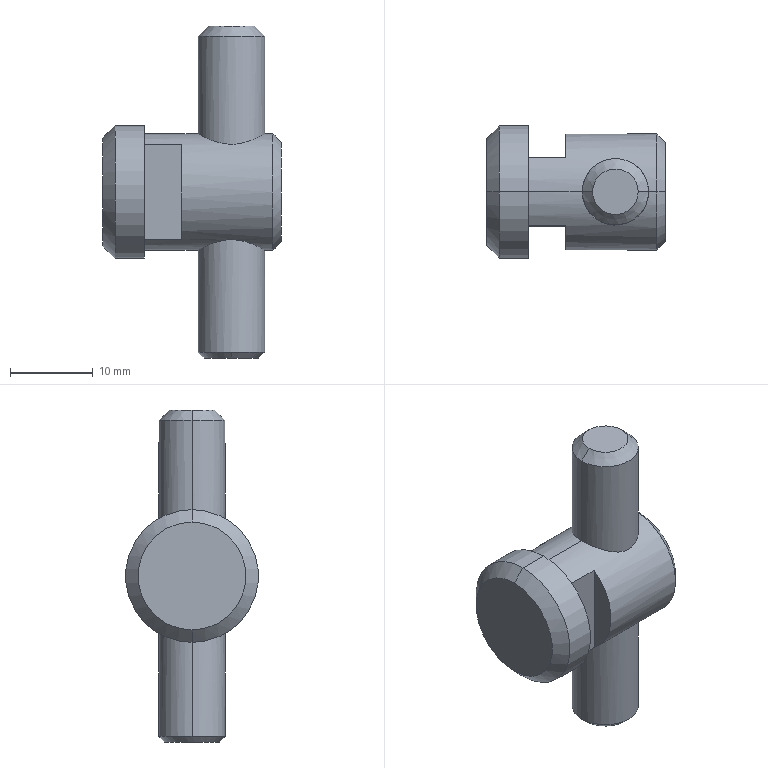Part | SolidWorks | features BaseBody 3, ICE 1 | 1 solid | 39 faces | box 21.5 x 16 x 40 mm | volume 4531 mm3 | plane 21 | cone 10 | cylinder 8 | commonest cylinder face diameters 8 x4 14 x2 16 x2
STEP:
#1=CARTESIAN_POINT('',(17.561,-2.765,31.125));
#2=VERTEX_POINT('',#1);
#3=CARTESIAN_POINT('',(25.561,-2.765,31.125));
#4=VERTEX_POINT('',#3);
#5=CARTESIAN_POINT('',(21.561,-2.765,31.125));
#6=DIRECTION('',(0.,0.,-1.));
#7=DIRECTION('',(-1.,0.,0.));
#8=AXIS2_PLACEMENT_3D('',#5,#6,#7);
#9=CIRCLE('',#8,4.);
#10=EDGE_CURVE('',#2,#4,#9,.T.);
#11=ORIENTED_EDGE('',*,*,#10,.T.);
#12=CARTESIAN_POINT('',(25.561,-2.765,19.375));
#13=VERTEX_POINT('',#12);
#14=CARTESIAN_POINT('',(25.561,-2.765,-18.37));
#15=DIRECTION('',(0.,0.,-1.));
#16=VECTOR('',#15,1000.);
#17=LINE('',#14,#16);
#18=EDGE_CURVE('',#4,#13,#17,.T.);
#19=ORIENTED_EDGE('',*,*,#18,.T.);
#20=CARTESIAN_POINT('',(17.561,-2.765,19.375));
#21=VERTEX_POINT('',#20);
#22=CARTESIAN_POINT('',(17.561,-2.765,19.375));
#23=CARTESIAN_POINT('',(17.561,-2.494,19.375));
#24=CARTESIAN_POINT('',(17.588,-2.229,19.359));
#25=CARTESIAN_POINT('',(17.694,-1.709,19.3));
#26=CARTESIAN_POINT('',(17.774,-1.452,19.255));
#27=CARTESIAN_POINT('',(17.977,-0.9687,19.145));
#28=CARTESIAN_POINT('',(18.101,-0.7408,19.08));
#29=CARTESIAN_POINT('',(18.392,-0.3103,18.934));
#30=CARTESIAN_POINT('',(18.556,-0.1123,18.856));
#31=CARTESIAN_POINT('',(18.917,0.2479,18.697));
#32=CARTESIAN_POINT('',(19.117,0.4123,18.615));
#33=CARTESIAN_POINT('',(19.544,0.6988,18.46));
#34=CARTESIAN_POINT('',(19.769,0.8207,18.388));
#35=CARTESIAN_POINT('',(20.247,1.022,18.263));
#36=CARTESIAN_POINT('',(20.503,1.102,18.21));
#37=CARTESIAN_POINT('',(21.023,1.208,18.139));
#38=CARTESIAN_POINT('',(21.289,1.235,18.12));
#39=CARTESIAN_POINT('',(21.831,1.235,18.12));
#40=CARTESIAN_POINT('',(22.096,1.208,18.139));
#41=CARTESIAN_POINT('',(22.616,1.103,18.21));
#42=CARTESIAN_POINT('',(22.872,1.023,18.263));
#43=CARTESIAN_POINT('',(23.352,0.8211,18.388));
#44=CARTESIAN_POINT('',(23.582,0.6969,18.461));
#45=CARTESIAN_POINT('',(24.009,0.4088,18.616));
#46=CARTESIAN_POINT('',(24.206,0.2466,18.697));
#47=CARTESIAN_POINT('',(24.568,-0.1149,18.857));
#48=CARTESIAN_POINT('',(24.734,-0.3159,18.937));
#49=CARTESIAN_POINT('',(25.021,-0.7423,19.08));
#50=CARTESIAN_POINT('',(25.145,-0.9692,19.145));
#51=CARTESIAN_POINT('',(25.298,-1.332,19.228));
#52=CARTESIAN_POINT('',(25.344,-1.458,19.253));
#53=CARTESIAN_POINT('',(25.422,-1.711,19.296));
#54=CARTESIAN_POINT('',(25.455,-1.84,19.315));
#55=CARTESIAN_POINT('',(25.534,-2.229,19.359));
#56=CARTESIAN_POINT('',(25.561,-2.494,19.375));
#57=CARTESIAN_POINT('',(25.561,-2.765,19.375));
#58=B_SPLINE_CURVE_WITH_KNOTS('',3,(#22,#23,#24,#25,#26,#27,#28,#29,#30,#31,#32,#33,#34,#35,#36,#37,#38,#39,#40,#41,#42,#43,#44,#45,#46,#47,#48,#49,#50,#51,#52,#53,#54,#55,#56,#57),.UNSPECIFIED.,.F.,.F.,(4,2,2,2,2,2,2,2,2,2,2,2,2,2,2,2,2,4),(0.,0.0007999,0.0016,0.0024,0.003199,0.003999,0.004799,0.005599,0.006399,0.007199,0.007999,0.008798,0.009598,0.0104,0.0112,0.0116,0.012,0.0128),.UNSPECIFIED.);
#59=EDGE_CURVE('',#21,#13,#58,.T.);
#60=ORIENTED_EDGE('',*,*,#59,.F.);
#61=CARTESIAN_POINT('',(17.561,-2.765,-18.37));
#62=DIRECTION('',(0.,0.,-1.));
#63=VECTOR('',#62,1000.);
#64=LINE('',#61,#63);
#65=EDGE_CURVE('',#2,#21,#64,.T.);
#66=ORIENTED_EDGE('',*,*,#65,.F.);
#67=EDGE_LOOP('',(#11,#19,#60,#66));
#68=FACE_OUTER_BOUND('',#67,.T.);
#69=CARTESIAN_POINT('',(21.561,-2.765,-18.37));
#70=DIRECTION('',(0.,0.,-1.));
#71=DIRECTION('',(-1.,0.,0.));
#72=AXIS2_PLACEMENT_3D('',#69,#70,#71);
#73=CYLINDRICAL_SURFACE('',#72,4.);
#74=ADVANCED_FACE('',(#68),#73,.T.);
#75=CARTESIAN_POINT('',(18.811,-2.765,32.375));
#76=VERTEX_POINT('',#75);
#77=CARTESIAN_POINT('',(24.311,-2.765,32.375));
#78=VERTEX_POINT('',#77);
#79=CARTESIAN_POINT('',(21.561,-2.765,32.375));
#80=DIRECTION('',(0.,0.,-1.));
#81=DIRECTION('',(-1.,0.,0.));
#82=AXIS2_PLACEMENT_3D('',#79,#80,#81);
#83=CIRCLE('',#82,2.75);
#84=EDGE_CURVE('',#76,#78,#83,.T.);
#85=ORIENTED_EDGE('',*,*,#84,.T.);
#86=CARTESIAN_POINT('',(25.561,-2.765,31.125));
#87=DIRECTION('',(0.7071,0.,-0.7071));
#88=VECTOR('',#87,1000.);
#89=LINE('',#86,#88);
#90=EDGE_CURVE('',#78,#4,#89,.T.);
#91=ORIENTED_EDGE('',*,*,#90,.T.);
#92=ORIENTED_EDGE('',*,*,#10,.F.);
#93=CARTESIAN_POINT('',(17.561,-2.765,31.125));
#94=DIRECTION('',(-0.7071,0.,-0.7071));
#95=VECTOR('',#94,1000.);
#96=LINE('',#93,#95);
#97=EDGE_CURVE('',#76,#2,#96,.T.);
#98=ORIENTED_EDGE('',*,*,#97,.F.);
#99=EDGE_LOOP('',(#85,#91,#92,#98));
#100=FACE_OUTER_BOUND('',#99,.T.);
#101=CARTESIAN_POINT('',(21.561,-2.765,31.125));
#102=DIRECTION('',(0.,0.,-1.));
#103=DIRECTION('',(-1.,0.,0.));
#104=AXIS2_PLACEMENT_3D('',#101,#102,#103);
#105=CONICAL_SURFACE('',#104,4.,0.7854);
#106=ADVANCED_FACE('',(#100),#105,.T.);
#107=CARTESIAN_POINT('',(26.561,-2.765,19.375));
#108=VERTEX_POINT('',#107);
#109=CARTESIAN_POINT('',(26.561,-2.765,5.375));
#110=VERTEX_POINT('',#109);
#111=CARTESIAN_POINT('',(26.561,-2.765,12.375));
#112=DIRECTION('',(-1.,0.,0.));
#113=DIRECTION('',(0.,0.,1.));
#114=AXIS2_PLACEMENT_3D('',#111,#112,#113);
#115=CIRCLE('',#114,7.);
#116=EDGE_CURVE('',#108,#110,#115,.T.);
#117=ORIENTED_EDGE('',*,*,#116,.T.);
#118=CARTESIAN_POINT('',(25.561,-2.765,5.375));
#119=VERTEX_POINT('',#118);
#120=CARTESIAN_POINT('',(27.561,-2.765,5.375));
#121=DIRECTION('',(-1.,0.,0.));
#122=VECTOR('',#121,1000.);
#123=LINE('',#120,#122);
#124=EDGE_CURVE('',#110,#119,#123,.T.);
#125=ORIENTED_EDGE('',*,*,#124,.T.);
#126=CARTESIAN_POINT('',(17.561,-2.765,5.375));
#127=VERTEX_POINT('',#126);
#128=CARTESIAN_POINT('',(25.561,-2.765,5.375));
#129=CARTESIAN_POINT('',(25.561,-2.494,5.375));
#130=CARTESIAN_POINT('',(25.534,-2.229,5.391));
#131=CARTESIAN_POINT('',(25.428,-1.709,5.45));
#132=CARTESIAN_POINT('',(25.348,-1.452,5.495));
#133=CARTESIAN_POINT('',(25.145,-0.9692,5.605));
#134=CARTESIAN_POINT('',(25.021,-0.7408,5.67));
#135=CARTESIAN_POINT('',(24.73,-0.3098,5.816));
#136=CARTESIAN_POINT('',(24.566,-0.1129,5.894));
#137=CARTESIAN_POINT('',(24.205,0.2473,6.053));
#138=CARTESIAN_POINT('',(24.005,0.412,6.135));
#139=CARTESIAN_POINT('',(23.58,0.6978,6.289));
#140=CARTESIAN_POINT('',(23.355,0.8199,6.361));
#141=CARTESIAN_POINT('',(22.876,1.022,6.486));
#142=CARTESIAN_POINT('',(22.62,1.101,6.539));
#143=CARTESIAN_POINT('',(22.101,1.207,6.611));
#144=CARTESIAN_POINT('',(21.833,1.235,6.63));
#145=CARTESIAN_POINT('',(21.294,1.235,6.631));
#146=CARTESIAN_POINT('',(21.029,1.209,6.612));
#147=CARTESIAN_POINT('',(20.508,1.103,6.54));
#148=CARTESIAN_POINT('',(20.253,1.024,6.488));
#149=CARTESIAN_POINT('',(19.773,0.8228,6.363));
#150=CARTESIAN_POINT('',(19.543,0.6984,6.29));
#151=CARTESIAN_POINT('',(19.116,0.4115,6.135));
#152=CARTESIAN_POINT('',(18.919,0.2497,6.054));
#153=CARTESIAN_POINT('',(18.556,-0.1119,5.894));
#154=CARTESIAN_POINT('',(18.391,-0.3121,5.815));
#155=CARTESIAN_POINT('',(18.103,-0.7374,5.671));
#156=CARTESIAN_POINT('',(17.979,-0.964,5.606));
#157=CARTESIAN_POINT('',(17.774,-1.449,5.495));
#158=CARTESIAN_POINT('',(17.695,-1.704,5.451));
#159=CARTESIAN_POINT('',(17.589,-2.224,5.391));
#160=CARTESIAN_POINT('',(17.561,-2.495,5.375));
#161=CARTESIAN_POINT('',(17.561,-2.765,5.375));
#162=B_SPLINE_CURVE_WITH_KNOTS('',3,(#128,#129,#130,#131,#132,#133,#134,#135,#136,#137,#138,#139,#140,#141,#142,#143,#144,#145,#146,#147,#148,#149,#150,#151,#152,#153,#154,#155,#156,#157,#158,#159,#160,#161),.UNSPECIFIED.,.F.,.F.,(4,2,2,2,2,2,2,2,2,2,2,2,2,2,2,2,4),(0.0128,0.0136,0.01439,0.01519,0.01599,0.01679,0.01759,0.01838,0.01918,0.01998,0.02078,0.02158,0.02238,0.02317,0.02397,0.02477,0.02557),.UNSPECIFIED.);
#163=EDGE_CURVE('',#119,#127,#162,.T.);
#164=ORIENTED_EDGE('',*,*,#163,.T.);
#165=CARTESIAN_POINT('',(11.061,-2.765,5.375));
#166=VERTEX_POINT('',#165);
#167=CARTESIAN_POINT('',(27.561,-2.765,5.375));
#168=DIRECTION('',(-1.,0.,0.));
#169=VECTOR('',#168,1000.);
#170=LINE('',#167,#169);
#171=EDGE_CURVE('',#127,#166,#170,.T.);
#172=ORIENTED_EDGE('',*,*,#171,.T.);
#173=CARTESIAN_POINT('',(11.061,1.335,6.701));
#174=VERTEX_POINT('',#173);
#175=CARTESIAN_POINT('',(11.061,-2.765,12.375));
#176=DIRECTION('',(1.,0.,0.));
#177=DIRECTION('',(0.,0.,1.));
#178=AXIS2_PLACEMENT_3D('',#175,#176,#177);
#179=CIRCLE('',#178,7.);
#180=EDGE_CURVE('',#166,#174,#179,.T.);
#181=ORIENTED_EDGE('',*,*,#180,.T.);
#182=CARTESIAN_POINT('',(15.561,1.335,6.701));
#183=VERTEX_POINT('',#182);
#184=CARTESIAN_POINT('',(27.561,1.335,6.701));
#185=DIRECTION('',(1.,0.,0.));
#186=VECTOR('',#185,1000.);
#187=LINE('',#184,#186);
#188=EDGE_CURVE('',#174,#183,#187,.T.);
#189=ORIENTED_EDGE('',*,*,#188,.T.);
#190=CARTESIAN_POINT('',(15.561,1.335,18.049));
#191=VERTEX_POINT('',#190);
#192=CARTESIAN_POINT('',(15.561,-2.765,12.375));
#193=DIRECTION('',(1.,0.,0.));
#194=DIRECTION('',(0.,0.,1.));
#195=AXIS2_PLACEMENT_3D('',#192,#193,#194);
#196=CIRCLE('',#195,7.);
#197=EDGE_CURVE('',#183,#191,#196,.T.);
#198=ORIENTED_EDGE('',*,*,#197,.T.);
#199=CARTESIAN_POINT('',(11.061,1.335,18.049));
#200=VERTEX_POINT('',#199);
#201=CARTESIAN_POINT('',(27.561,1.335,18.049));
#202=DIRECTION('',(-1.,0.,0.));
#203=VECTOR('',#202,1000.);
#204=LINE('',#201,#203);
#205=EDGE_CURVE('',#191,#200,#204,.T.);
#206=ORIENTED_EDGE('',*,*,#205,.T.);
#207=CARTESIAN_POINT('',(11.061,-2.765,19.375));
#208=VERTEX_POINT('',#207);
#209=CARTESIAN_POINT('',(11.061,-2.765,12.375));
#210=DIRECTION('',(1.,0.,0.));
#211=DIRECTION('',(0.,0.,1.));
#212=AXIS2_PLACEMENT_3D('',#209,#210,#211);
#213=CIRCLE('',#212,7.);
#214=EDGE_CURVE('',#200,#208,#213,.T.);
#215=ORIENTED_EDGE('',*,*,#214,.T.);
#216=CARTESIAN_POINT('',(27.561,-2.765,19.375));
#217=DIRECTION('',(-1.,0.,0.));
#218=VECTOR('',#217,1000.);
#219=LINE('',#216,#218);
#220=EDGE_CURVE('',#21,#208,#219,.T.);
#221=ORIENTED_EDGE('',*,*,#220,.F.);
#222=ORIENTED_EDGE('',*,*,#59,.T.);
#223=CARTESIAN_POINT('',(27.561,-2.765,19.375));
#224=DIRECTION('',(-1.,0.,0.));
#225=VECTOR('',#224,1000.);
#226=LINE('',#223,#225);
#227=EDGE_CURVE('',#108,#13,#226,.T.);
#228=ORIENTED_EDGE('',*,*,#227,.F.);
#229=EDGE_LOOP('',(#117,#125,#164,#172,#181,#189,#198,#206,#215,#221,#222,#228));
#230=FACE_OUTER_BOUND('',#229,.T.);
#231=CARTESIAN_POINT('',(27.561,-2.765,12.375));
#232=DIRECTION('',(-1.,0.,0.));
#233=DIRECTION('',(0.,0.,1.));
#234=AXIS2_PLACEMENT_3D('',#231,#232,#233);
#235=CYLINDRICAL_SURFACE('',#234,7.);
#236=ADVANCED_FACE('',(#230),#235,.T.);
#237=CARTESIAN_POINT('',(27.561,-2.765,18.375));
#238=VERTEX_POINT('',#237);
#239=CARTESIAN_POINT('',(27.561,-2.765,6.375));
#240=VERTEX_POINT('',#239);
#241=CARTESIAN_POINT('',(27.561,-2.765,12.375));
#242=DIRECTION('',(-1.,0.,0.));
#243=DIRECTION('',(0.,0.,1.));
#244=AXIS2_PLACEMENT_3D('',#241,#242,#243);
#245=CIRCLE('',#244,6.);
#246=EDGE_CURVE('',#238,#240,#245,.T.);
#247=ORIENTED_EDGE('',*,*,#246,.T.);
#248=CARTESIAN_POINT('',(26.561,-2.765,5.375));
#249=DIRECTION('',(-0.7071,0.,-0.7071));
#250=VECTOR('',#249,1000.);
#251=LINE('',#248,#250);
#252=EDGE_CURVE('',#240,#110,#251,.T.);
#253=ORIENTED_EDGE('',*,*,#252,.T.);
#254=ORIENTED_EDGE('',*,*,#116,.F.);
#255=CARTESIAN_POINT('',(26.561,-2.765,19.375));
#256=DIRECTION('',(-0.7071,0.,0.7071));
#257=VECTOR('',#256,1000.);
#258=LINE('',#255,#257);
#259=EDGE_CURVE('',#238,#108,#258,.T.);
#260=ORIENTED_EDGE('',*,*,#259,.F.);
#261=EDGE_LOOP('',(#247,#253,#254,#260));
#262=FACE_OUTER_BOUND('',#261,.T.);
#263=CARTESIAN_POINT('',(26.561,-2.765,12.375));
#264=DIRECTION('',(-1.,0.,0.));
#265=DIRECTION('',(0.,0.,1.));
#266=AXIS2_PLACEMENT_3D('',#263,#264,#265);
#267=CONICAL_SURFACE('',#266,7.,0.7854);
#268=ADVANCED_FACE('',(#262),#267,.T.);
#269=CARTESIAN_POINT('',(11.061,-2.765,4.375));
#270=VERTEX_POINT('',#269);
#271=CARTESIAN_POINT('',(11.061,-2.765,20.375));
#272=VERTEX_POINT('',#271);
#273=CARTESIAN_POINT('',(11.061,-2.765,12.375));
#274=DIRECTION('',(1.,0.,0.));
#275=DIRECTION('',(0.,0.,1.));
#276=AXIS2_PLACEMENT_3D('',#273,#274,#275);
#277=CIRCLE('',#276,8.);
#278=EDGE_CURVE('',#270,#272,#277,.T.);
#279=ORIENTED_EDGE('',*,*,#278,.F.);
#280=CARTESIAN_POINT('',(7.561,-2.765,4.375));
#281=VERTEX_POINT('',#280);
#282=CARTESIAN_POINT('',(11.061,-2.765,4.375));
#283=DIRECTION('',(-1.,0.,0.));
#284=VECTOR('',#283,1000.);
#285=LINE('',#282,#284);
#286=EDGE_CURVE('',#270,#281,#285,.T.);
#287=ORIENTED_EDGE('',*,*,#286,.T.);
#288=CARTESIAN_POINT('',(7.561,-2.765,20.375));
#289=VERTEX_POINT('',#288);
#290=CARTESIAN_POINT('',(7.561,-2.765,12.375));
#291=DIRECTION('',(1.,0.,0.));
#292=DIRECTION('',(0.,0.,1.));
#293=AXIS2_PLACEMENT_3D('',#290,#291,#292);
#294=CIRCLE('',#293,8.);
#295=EDGE_CURVE('',#281,#289,#294,.T.);
#296=ORIENTED_EDGE('',*,*,#295,.T.);
#297=CARTESIAN_POINT('',(11.061,-2.765,20.375));
#298=DIRECTION('',(-1.,0.,0.));
#299=VECTOR('',#298,1000.);
#300=LINE('',#297,#299);
#301=EDGE_CURVE('',#272,#289,#300,.T.);
#302=ORIENTED_EDGE('',*,*,#301,.F.);
#303=EDGE_LOOP('',(#279,#287,#296,#302));
#304=FACE_OUTER_BOUND('',#303,.T.);
#305=CARTESIAN_POINT('',(11.061,-2.765,12.375));
#306=DIRECTION('',(-1.,0.,0.));
#307=DIRECTION('',(0.,0.,1.));
#308=AXIS2_PLACEMENT_3D('',#305,#306,#307);
#309=CYLINDRICAL_SURFACE('',#308,8.);
#310=ADVANCED_FACE('',(#304),#309,.T.);
#311=CARTESIAN_POINT('',(6.061,-2.765,5.875));
#312=VERTEX_POINT('',#311);
#313=CARTESIAN_POINT('',(6.061,-2.765,18.875));
#314=VERTEX_POINT('',#313);
#315=CARTESIAN_POINT('',(6.061,-2.765,12.375));
#316=DIRECTION('',(1.,0.,0.));
#317=DIRECTION('',(0.,0.,-1.));
#318=AXIS2_PLACEMENT_3D('',#315,#316,#317);
#319=CIRCLE('',#318,6.5);
#320=EDGE_CURVE('',#312,#314,#319,.T.);
#321=ORIENTED_EDGE('',*,*,#320,.T.);
#322=CARTESIAN_POINT('',(7.561,-2.765,20.375));
#323=DIRECTION('',(0.7071,0.,0.7071));
#324=VECTOR('',#323,1000.);
#325=LINE('',#322,#324);
#326=EDGE_CURVE('',#314,#289,#325,.T.);
#327=ORIENTED_EDGE('',*,*,#326,.T.);
#328=ORIENTED_EDGE('',*,*,#295,.F.);
#329=CARTESIAN_POINT('',(7.561,-2.765,4.375));
#330=DIRECTION('',(0.7071,0.,-0.7071));
#331=VECTOR('',#330,1000.);
#332=LINE('',#329,#331);
#333=EDGE_CURVE('',#312,#281,#332,.T.);
#334=ORIENTED_EDGE('',*,*,#333,.F.);
#335=EDGE_LOOP('',(#321,#327,#328,#334));
#336=FACE_OUTER_BOUND('',#335,.T.);
#337=CARTESIAN_POINT('',(7.561,-2.765,12.375));
#338=DIRECTION('',(1.,0.,0.));
#339=DIRECTION('',(0.,0.,-1.));
#340=AXIS2_PLACEMENT_3D('',#337,#338,#339);
#341=CONICAL_SURFACE('',#340,8.,0.7854);
#342=ADVANCED_FACE('',(#336),#341,.T.);
#343=ORIENTED_EDGE('',*,*,#163,.F.);
#344=CARTESIAN_POINT('',(25.561,-2.765,-6.948));
#345=VERTEX_POINT('',#344);
#346=CARTESIAN_POINT('',(25.561,-2.765,-18.37));
#347=DIRECTION('',(0.,0.,-1.));
#348=VECTOR('',#347,1000.);
#349=LINE('',#346,#348);
#350=EDGE_CURVE('',#119,#345,#349,.T.);
#351=ORIENTED_EDGE('',*,*,#350,.T.);
#352=CARTESIAN_POINT('',(21.561,1.235,-6.948));
#353=VERTEX_POINT('',#352);
#354=CARTESIAN_POINT('',(21.561,-2.765,-6.948));
#355=DIRECTION('',(0.,0.,1.));
#356=DIRECTION('',(-1.,0.,0.));
#357=AXIS2_PLACEMENT_3D('',#354,#355,#356);
#358=CIRCLE('',#357,4.);
#359=EDGE_CURVE('',#345,#353,#358,.T.);
#360=ORIENTED_EDGE('',*,*,#359,.T.);
#361=CARTESIAN_POINT('',(17.561,-2.765,-6.948));
#362=VERTEX_POINT('',#361);
#363=CARTESIAN_POINT('',(21.561,-2.765,-6.948));
#364=DIRECTION('',(0.,0.,1.));
#365=DIRECTION('',(-1.,0.,0.));
#366=AXIS2_PLACEMENT_3D('',#363,#364,#365);
#367=CIRCLE('',#366,4.);
#368=EDGE_CURVE('',#353,#362,#367,.T.);
#369=ORIENTED_EDGE('',*,*,#368,.T.);
#370=CARTESIAN_POINT('',(17.561,-2.765,-18.37));
#371=DIRECTION('',(0.,0.,-1.));
#372=VECTOR('',#371,1000.);
#373=LINE('',#370,#372);
#374=EDGE_CURVE('',#127,#362,#373,.T.);
#375=ORIENTED_EDGE('',*,*,#374,.F.);
#376=EDGE_LOOP('',(#343,#351,#360,#369,#375));
#377=FACE_OUTER_BOUND('',#376,.T.);
#378=CARTESIAN_POINT('',(21.561,-2.765,-18.37));
#379=DIRECTION('',(0.,0.,-1.));
#380=DIRECTION('',(-1.,0.,0.));
#381=AXIS2_PLACEMENT_3D('',#378,#379,#380);
#382=CYLINDRICAL_SURFACE('',#381,4.);
#383=ADVANCED_FACE('',(#377),#382,.T.);
#384=CARTESIAN_POINT('',(21.561,-6.088,-7.625));
#385=VERTEX_POINT('',#384);
#386=CARTESIAN_POINT('',(21.561,0.5587,-7.625));
#387=VERTEX_POINT('',#386);
#388=CARTESIAN_POINT('',(21.561,-2.765,-7.625));
#389=DIRECTION('',(0.,0.,1.));
#390=DIRECTION('',(0.,-1.,0.));
#391=AXIS2_PLACEMENT_3D('',#388,#389,#390);
#392=CIRCLE('',#391,3.323);
#393=EDGE_CURVE('',#385,#387,#392,.T.);
#394=ORIENTED_EDGE('',*,*,#393,.T.);
#395=CARTESIAN_POINT('',(21.561,1.235,-6.949));
#396=DIRECTION('',(0.,0.7071,0.7071));
#397=VECTOR('',#396,1000.);
#398=LINE('',#395,#397);
#399=EDGE_CURVE('',#387,#353,#398,.T.);
#400=ORIENTED_EDGE('',*,*,#399,.T.);
#401=ORIENTED_EDGE('',*,*,#359,.F.);
#402=CARTESIAN_POINT('',(21.561,-6.765,-6.948));
#403=VERTEX_POINT('',#402);
#404=CARTESIAN_POINT('',(21.561,-2.765,-6.948));
#405=DIRECTION('',(0.,0.,1.));
#406=DIRECTION('',(-1.,0.,0.));
#407=AXIS2_PLACEMENT_3D('',#404,#405,#406);
#408=CIRCLE('',#407,4.);
#409=EDGE_CURVE('',#403,#345,#408,.T.);
#410=ORIENTED_EDGE('',*,*,#409,.F.);
#411=CARTESIAN_POINT('',(21.561,-6.765,-6.949));
#412=DIRECTION('',(0.,-0.7071,0.7071));
#413=VECTOR('',#412,1000.);
#414=LINE('',#411,#413);
#415=EDGE_CURVE('',#385,#403,#414,.T.);
#416=ORIENTED_EDGE('',*,*,#415,.F.);
#417=EDGE_LOOP('',(#394,#400,#401,#410,#416));
#418=FACE_OUTER_BOUND('',#417,.T.);
#419=CARTESIAN_POINT('',(21.561,-2.765,-6.949));
#420=DIRECTION('',(0.,0.,1.));
#421=DIRECTION('',(0.,-1.,0.));
#422=AXIS2_PLACEMENT_3D('',#419,#420,#421);
#423=CONICAL_SURFACE('',#422,4.,0.7854);
#424=ADVANCED_FACE('',(#418),#423,.T.);
#425=CARTESIAN_POINT('',(21.561,-2.765,-3.47));
#426=VERTEX_POINT('',#425);
#427=CARTESIAN_POINT('',(21.561,-0.7648,-4.625));
#428=VERTEX_POINT('',#427);
#429=CARTESIAN_POINT('',(21.561,-0.7648,-4.625));
#430=DIRECTION('',(0.,0.866,-0.5));
#431=VECTOR('',#430,1000.);
#432=LINE('',#429,#431);
#433=EDGE_CURVE('',#426,#428,#432,.T.);
#434=ORIENTED_EDGE('',*,*,#433,.F.);
#435=CARTESIAN_POINT('',(21.561,-4.765,-4.625));
#436=VERTEX_POINT('',#435);
#437=CARTESIAN_POINT('',(21.561,-4.765,-4.625));
#438=DIRECTION('',(0.,-0.866,-0.5));
#439=VECTOR('',#438,1000.);
#440=LINE('',#437,#439);
#441=EDGE_CURVE('',#426,#436,#440,.T.);
#442=ORIENTED_EDGE('',*,*,#441,.T.);
#443=CARTESIAN_POINT('',(20.212,-4.242,-4.625));
#444=VERTEX_POINT('',#443);
#445=CARTESIAN_POINT('',(21.561,-2.765,-4.625));
#446=DIRECTION('',(0.,0.,-1.));
#447=DIRECTION('',(0.,1.,0.));
#448=AXIS2_PLACEMENT_3D('',#445,#446,#447);
#449=CIRCLE('',#448,2.);
#450=EDGE_CURVE('',#436,#444,#449,.T.);
#451=ORIENTED_EDGE('',*,*,#450,.T.);
#452=CARTESIAN_POINT('',(19.607,-2.335,-4.625));
#453=VERTEX_POINT('',#452);
#454=CARTESIAN_POINT('',(21.561,-2.765,-4.625));
#455=DIRECTION('',(0.,0.,1.));
#456=DIRECTION('',(0.,1.,0.));
#457=AXIS2_PLACEMENT_3D('',#454,#455,#456);
#458=CIRCLE('',#457,2.);
#459=EDGE_CURVE('',#453,#444,#458,.T.);
#460=ORIENTED_EDGE('',*,*,#459,.F.);
#461=CARTESIAN_POINT('',(20.956,-0.8585,-4.625));
#462=VERTEX_POINT('',#461);
#463=CARTESIAN_POINT('',(21.561,-2.765,-4.625));
#464=DIRECTION('',(0.,0.,1.));
#465=DIRECTION('',(0.,1.,0.));
#466=AXIS2_PLACEMENT_3D('',#463,#464,#465);
#467=CIRCLE('',#466,2.);
#468=EDGE_CURVE('',#462,#453,#467,.T.);
#469=ORIENTED_EDGE('',*,*,#468,.F.);
#470=CARTESIAN_POINT('',(21.561,-2.765,-4.625));
#471=DIRECTION('',(0.,0.,1.));
#472=DIRECTION('',(0.,1.,0.));
#473=AXIS2_PLACEMENT_3D('',#470,#471,#472);
#474=CIRCLE('',#473,2.);
#475=EDGE_CURVE('',#428,#462,#474,.T.);
#476=ORIENTED_EDGE('',*,*,#475,.F.);
#477=EDGE_LOOP('',(#434,#442,#451,#460,#469,#476));
#478=FACE_OUTER_BOUND('',#477,.T.);
#479=CARTESIAN_POINT('',(21.561,-2.765,-4.625));
#480=DIRECTION('',(0.,0.,-1.));
#481=DIRECTION('',(0.,1.,0.));
#482=AXIS2_PLACEMENT_3D('',#479,#480,#481);
#483=CONICAL_SURFACE('',#482,2.,1.047);
#484=ADVANCED_FACE('',(#478),#483,.F.);
#485=ORIENTED_EDGE('',*,*,#350,.F.);
#486=CARTESIAN_POINT('',(17.561,-2.765,5.375));
#487=CARTESIAN_POINT('',(17.561,-3.036,5.375));
#488=CARTESIAN_POINT('',(17.588,-3.301,5.391));
#489=CARTESIAN_POINT('',(17.694,-3.821,5.45));
#490=CARTESIAN_POINT('',(17.774,-4.078,5.495));
#491=CARTESIAN_POINT('',(17.977,-4.561,5.605));
#492=CARTESIAN_POINT('',(18.101,-4.789,5.67));
#493=CARTESIAN_POINT('',(18.392,-5.219,5.816));
#494=CARTESIAN_POINT('',(18.556,-5.417,5.894));
#495=CARTESIAN_POINT('',(18.917,-5.778,6.053));
#496=CARTESIAN_POINT('',(19.117,-5.942,6.135));
#497=CARTESIAN_POINT('',(19.544,-6.228,6.29));
#498=CARTESIAN_POINT('',(19.769,-6.35,6.362));
#499=CARTESIAN_POINT('',(20.247,-6.552,6.487));
#500=CARTESIAN_POINT('',(20.503,-6.631,6.54));
#501=CARTESIAN_POINT('',(21.023,-6.737,6.611));
#502=CARTESIAN_POINT('',(21.289,-6.765,6.63));
#503=CARTESIAN_POINT('',(21.831,-6.765,6.63));
#504=CARTESIAN_POINT('',(22.096,-6.738,6.611));
#505=CARTESIAN_POINT('',(22.616,-6.632,6.54));
#506=CARTESIAN_POINT('',(22.872,-6.553,6.487));
#507=CARTESIAN_POINT('',(23.352,-6.351,6.362));
#508=CARTESIAN_POINT('',(23.582,-6.227,6.289));
#509=CARTESIAN_POINT('',(24.009,-5.938,6.134));
#510=CARTESIAN_POINT('',(24.206,-5.776,6.053));
#511=CARTESIAN_POINT('',(24.568,-5.415,5.893));
#512=CARTESIAN_POINT('',(24.734,-5.214,5.813));
#513=CARTESIAN_POINT('',(25.021,-4.787,5.67));
#514=CARTESIAN_POINT('',(25.145,-4.56,5.605));
#515=CARTESIAN_POINT('',(25.298,-4.197,5.522));
#516=CARTESIAN_POINT('',(25.344,-4.072,5.497));
#517=CARTESIAN_POINT('',(25.422,-3.818,5.454));
#518=CARTESIAN_POINT('',(25.455,-3.69,5.435));
#519=CARTESIAN_POINT('',(25.534,-3.301,5.391));
#520=CARTESIAN_POINT('',(25.561,-3.036,5.375));
#521=CARTESIAN_POINT('',(25.561,-2.765,5.375));
#522=B_SPLINE_CURVE_WITH_KNOTS('',3,(#486,#487,#488,#489,#490,#491,#492,#493,#494,#495,#496,#497,#498,#499,#500,#501,#502,#503,#504,#505,#506,#507,#508,#509,#510,#511,#512,#513,#514,#515,#516,#517,#518,#519,#520,#521),.UNSPECIFIED.,.F.,.F.,(4,2,2,2,2,2,2,2,2,2,2,2,2,2,2,2,2,4),(0.,0.0007999,0.0016,0.0024,0.003199,0.003999,0.004799,0.005599,0.006399,0.007199,0.007999,0.008798,0.009598,0.0104,0.0112,0.0116,0.012,0.0128),.UNSPECIFIED.);
#523=EDGE_CURVE('',#127,#119,#522,.T.);
#524=ORIENTED_EDGE('',*,*,#523,.F.);
#525=ORIENTED_EDGE('',*,*,#374,.T.);
#526=CARTESIAN_POINT('',(21.561,-2.765,-6.948));
#527=DIRECTION('',(0.,0.,1.));
#528=DIRECTION('',(-1.,0.,0.));
#529=AXIS2_PLACEMENT_3D('',#526,#527,#528);
#530=CIRCLE('',#529,4.);
#531=EDGE_CURVE('',#362,#403,#530,.T.);
#532=ORIENTED_EDGE('',*,*,#531,.T.);
#533=ORIENTED_EDGE('',*,*,#409,.T.);
#534=EDGE_LOOP('',(#485,#524,#525,#532,#533));
#535=FACE_OUTER_BOUND('',#534,.T.);
#536=CARTESIAN_POINT('',(21.561,-2.765,-18.37));
#537=DIRECTION('',(0.,0.,-1.));
#538=DIRECTION('',(-1.,0.,0.));
#539=AXIS2_PLACEMENT_3D('',#536,#537,#538);
#540=CYLINDRICAL_SURFACE('',#539,4.);
#541=ADVANCED_FACE('',(#535),#540,.T.);
#542=ORIENTED_EDGE('',*,*,#399,.F.);
#543=CARTESIAN_POINT('',(21.561,-2.765,-7.625));
#544=DIRECTION('',(0.,0.,1.));
#545=DIRECTION('',(0.,-1.,0.));
#546=AXIS2_PLACEMENT_3D('',#543,#544,#545);
#547=CIRCLE('',#546,3.323);
#548=EDGE_CURVE('',#387,#385,#547,.T.);
#549=ORIENTED_EDGE('',*,*,#548,.T.);
#550=ORIENTED_EDGE('',*,*,#415,.T.);
#551=ORIENTED_EDGE('',*,*,#531,.F.);
#552=ORIENTED_EDGE('',*,*,#368,.F.);
#553=EDGE_LOOP('',(#542,#549,#550,#551,#552));
#554=FACE_OUTER_BOUND('',#553,.T.);
#555=CARTESIAN_POINT('',(21.561,-2.765,-6.949));
#556=DIRECTION('',(0.,0.,1.));
#557=DIRECTION('',(0.,-1.,0.));
#558=AXIS2_PLACEMENT_3D('',#555,#556,#557);
#559=CONICAL_SURFACE('',#558,4.,0.7854);
#560=ADVANCED_FACE('',(#554),#559,.T.);
#561=CARTESIAN_POINT('',(22.057,-0.5093,-7.625));
#562=VERTEX_POINT('',#561);
#563=CARTESIAN_POINT('',(23.762,-2.066,-7.625));
#564=VERTEX_POINT('',#563);
#565=CARTESIAN_POINT('',(22.057,-0.5093,-7.625));
#566=DIRECTION('',(0.7385,-0.6743,0.));
#567=VECTOR('',#566,1000.);
#568=LINE('',#565,#567);
#569=EDGE_CURVE('',#562,#564,#568,.T.);
#570=ORIENTED_EDGE('',*,*,#569,.F.);
#571=CARTESIAN_POINT('',(19.855,-1.208,-7.625));
#572=VERTEX_POINT('',#571);
#573=CARTESIAN_POINT('',(19.855,-1.208,-7.625));
#574=DIRECTION('',(0.9532,0.3024,0.));
#575=VECTOR('',#574,1000.);
#576=LINE('',#573,#575);
#577=EDGE_CURVE('',#572,#562,#576,.T.);
#578=ORIENTED_EDGE('',*,*,#577,.F.);
#579=CARTESIAN_POINT('',(19.36,-3.463,-7.625));
#580=VERTEX_POINT('',#579);
#581=CARTESIAN_POINT('',(19.36,-3.463,-7.625));
#582=DIRECTION('',(0.2147,0.9767,0.));
#583=VECTOR('',#582,1000.);
#584=LINE('',#581,#583);
#585=EDGE_CURVE('',#580,#572,#584,.T.);
#586=ORIENTED_EDGE('',*,*,#585,.F.);
#587=CARTESIAN_POINT('',(21.065,-5.02,-7.625));
#588=VERTEX_POINT('',#587);
#589=CARTESIAN_POINT('',(21.065,-5.02,-7.625));
#590=DIRECTION('',(-0.7385,0.6743,0.));
#591=VECTOR('',#590,1000.);
#592=LINE('',#589,#591);
#593=EDGE_CURVE('',#588,#580,#592,.T.);
#594=ORIENTED_EDGE('',*,*,#593,.F.);
#595=CARTESIAN_POINT('',(23.266,-4.322,-7.625));
#596=VERTEX_POINT('',#595);
#597=CARTESIAN_POINT('',(23.266,-4.322,-7.625));
#598=DIRECTION('',(-0.9532,-0.3024,0.));
#599=VECTOR('',#598,1000.);
#600=LINE('',#597,#599);
#601=EDGE_CURVE('',#596,#588,#600,.T.);
#602=ORIENTED_EDGE('',*,*,#601,.F.);
#603=CARTESIAN_POINT('',(23.762,-2.066,-7.625));
#604=DIRECTION('',(-0.2147,-0.9767,0.));
#605=VECTOR('',#604,1000.);
#606=LINE('',#603,#605);
#607=EDGE_CURVE('',#564,#596,#606,.T.);
#608=ORIENTED_EDGE('',*,*,#607,.F.);
#609=EDGE_LOOP('',(#570,#578,#586,#594,#602,#608));
#610=FACE_BOUND('',#609,.T.);
#611=ORIENTED_EDGE('',*,*,#393,.F.);
#612=ORIENTED_EDGE('',*,*,#548,.F.);
#613=EDGE_LOOP('',(#611,#612));
#614=FACE_OUTER_BOUND('',#613,.T.);
#615=CARTESIAN_POINT('',(19.32,-5.219,-7.625));
#616=DIRECTION('',(0.,0.,1.));
#617=DIRECTION('',(1.,0.,0.));
#618=AXIS2_PLACEMENT_3D('',#615,#616,#617);
#619=PLANE('',#618);
#620=ADVANCED_FACE('',(#610,#614),#619,.F.);
#621=CARTESIAN_POINT('',(23.266,-4.322,-4.625));
#622=VERTEX_POINT('',#621);
#623=CARTESIAN_POINT('',(23.514,-3.194,-4.625));
#624=VERTEX_POINT('',#623);
#625=CARTESIAN_POINT('',(23.266,-4.322,-4.625));
#626=DIRECTION('',(0.2147,0.9767,0.));
#627=VECTOR('',#626,1000.);
#628=LINE('',#625,#627);
#629=EDGE_CURVE('',#622,#624,#628,.T.);
#630=ORIENTED_EDGE('',*,*,#629,.T.);
#631=CARTESIAN_POINT('',(23.762,-2.066,-4.625));
#632=VERTEX_POINT('',#631);
#633=CARTESIAN_POINT('',(23.514,-3.194,-4.625));
#634=DIRECTION('',(0.2147,0.9767,0.));
#635=VECTOR('',#634,1000.);
#636=LINE('',#633,#635);
#637=EDGE_CURVE('',#624,#632,#636,.T.);
#638=ORIENTED_EDGE('',*,*,#637,.T.);
#639=CARTESIAN_POINT('',(23.762,-2.066,-4.625));
#640=DIRECTION('',(0.,0.,1.));
#641=VECTOR('',#640,1000.);
#642=LINE('',#639,#641);
#643=EDGE_CURVE('',#564,#632,#642,.T.);
#644=ORIENTED_EDGE('',*,*,#643,.F.);
#645=ORIENTED_EDGE('',*,*,#607,.T.);
#646=CARTESIAN_POINT('',(23.266,-4.322,-4.625));
#647=DIRECTION('',(0.,0.,-1.));
#648=VECTOR('',#647,1000.);
#649=LINE('',#646,#648);
#650=EDGE_CURVE('',#622,#596,#649,.T.);
#651=ORIENTED_EDGE('',*,*,#650,.F.);
#652=EDGE_LOOP('',(#630,#638,#644,#645,#651));
#653=FACE_OUTER_BOUND('',#652,.T.);
#654=CARTESIAN_POINT('',(23.762,-2.066,-4.625));
#655=DIRECTION('',(0.9767,-0.2147,0.));
#656=DIRECTION('',(0.2147,0.9767,0.));
#657=AXIS2_PLACEMENT_3D('',#654,#655,#656);
#658=PLANE('',#657);
#659=ADVANCED_FACE('',(#653),#658,.F.);
#660=CARTESIAN_POINT('',(22.909,-1.288,-4.625));
#661=VERTEX_POINT('',#660);
#662=CARTESIAN_POINT('',(23.762,-2.066,-4.625));
#663=DIRECTION('',(-0.7385,0.6743,0.));
#664=VECTOR('',#663,1000.);
#665=LINE('',#662,#664);
#666=EDGE_CURVE('',#632,#661,#665,.T.);
#667=ORIENTED_EDGE('',*,*,#666,.T.);
#668=CARTESIAN_POINT('',(22.057,-0.5093,-4.625));
#669=VERTEX_POINT('',#668);
#670=CARTESIAN_POINT('',(22.909,-1.288,-4.625));
#671=DIRECTION('',(-0.7385,0.6743,0.));
#672=VECTOR('',#671,1000.);
#673=LINE('',#670,#672);
#674=EDGE_CURVE('',#661,#669,#673,.T.);
#675=ORIENTED_EDGE('',*,*,#674,.T.);
#676=CARTESIAN_POINT('',(22.057,-0.5093,-4.625));
#677=DIRECTION('',(0.,0.,1.));
#678=VECTOR('',#677,1000.);
#679=LINE('',#676,#678);
#680=EDGE_CURVE('',#562,#669,#679,.T.);
#681=ORIENTED_EDGE('',*,*,#680,.F.);
#682=ORIENTED_EDGE('',*,*,#569,.T.);
#683=ORIENTED_EDGE('',*,*,#643,.T.);
#684=EDGE_LOOP('',(#667,#675,#681,#682,#683));
#685=FACE_OUTER_BOUND('',#684,.T.);
#686=CARTESIAN_POINT('',(22.057,-0.5093,-4.625));
#687=DIRECTION('',(0.6743,0.7385,0.));
#688=DIRECTION('',(-0.7385,0.6743,0.));
#689=AXIS2_PLACEMENT_3D('',#686,#687,#688);
#690=PLANE('',#689);
#691=ADVANCED_FACE('',(#685),#690,.F.);
#692=CARTESIAN_POINT('',(22.057,-0.5093,-4.625));
#693=DIRECTION('',(-0.9532,-0.3024,0.));
#694=VECTOR('',#693,1000.);
#695=LINE('',#692,#694);
#696=EDGE_CURVE('',#669,#462,#695,.T.);
#697=ORIENTED_EDGE('',*,*,#696,.T.);
#698=CARTESIAN_POINT('',(19.855,-1.208,-4.625));
#699=VERTEX_POINT('',#698);
#700=CARTESIAN_POINT('',(20.956,-0.8585,-4.625));
#701=DIRECTION('',(-0.9532,-0.3024,0.));
#702=VECTOR('',#701,1000.);
#703=LINE('',#700,#702);
#704=EDGE_CURVE('',#462,#699,#703,.T.);
#705=ORIENTED_EDGE('',*,*,#704,.T.);
#706=CARTESIAN_POINT('',(19.855,-1.208,-4.625));
#707=DIRECTION('',(0.,0.,1.));
#708=VECTOR('',#707,1000.);
#709=LINE('',#706,#708);
#710=EDGE_CURVE('',#572,#699,#709,.T.);
#711=ORIENTED_EDGE('',*,*,#710,.F.);
#712=ORIENTED_EDGE('',*,*,#577,.T.);
#713=ORIENTED_EDGE('',*,*,#680,.T.);
#714=EDGE_LOOP('',(#697,#705,#711,#712,#713));
#715=FACE_OUTER_BOUND('',#714,.T.);
#716=CARTESIAN_POINT('',(19.855,-1.208,-4.625));
#717=DIRECTION('',(-0.3024,0.9532,0.));
#718=DIRECTION('',(-0.9532,-0.3024,0.));
#719=AXIS2_PLACEMENT_3D('',#716,#717,#718);
#720=PLANE('',#719);
#721=ADVANCED_FACE('',(#715),#720,.F.);
#722=CARTESIAN_POINT('',(19.855,-1.208,-4.625));
#723=DIRECTION('',(-0.2147,-0.9767,0.));
#724=VECTOR('',#723,1000.);
#725=LINE('',#722,#724);
#726=EDGE_CURVE('',#699,#453,#725,.T.);
#727=ORIENTED_EDGE('',*,*,#726,.T.);
#728=CARTESIAN_POINT('',(19.36,-3.463,-4.625));
#729=VERTEX_POINT('',#728);
#730=CARTESIAN_POINT('',(19.607,-2.335,-4.625));
#731=DIRECTION('',(-0.2147,-0.9767,0.));
#732=VECTOR('',#731,1000.);
#733=LINE('',#730,#732);
#734=EDGE_CURVE('',#453,#729,#733,.T.);
#735=ORIENTED_EDGE('',*,*,#734,.T.);
#736=CARTESIAN_POINT('',(19.36,-3.463,-4.625));
#737=DIRECTION('',(0.,0.,1.));
#738=VECTOR('',#737,1000.);
#739=LINE('',#736,#738);
#740=EDGE_CURVE('',#580,#729,#739,.T.);
#741=ORIENTED_EDGE('',*,*,#740,.F.);
#742=ORIENTED_EDGE('',*,*,#585,.T.);
#743=ORIENTED_EDGE('',*,*,#710,.T.);
#744=EDGE_LOOP('',(#727,#735,#741,#742,#743));
#745=FACE_OUTER_BOUND('',#744,.T.);
#746=CARTESIAN_POINT('',(19.36,-3.463,-4.625));
#747=DIRECTION('',(-0.9767,0.2147,0.));
#748=DIRECTION('',(-0.2147,-0.9767,0.));
#749=AXIS2_PLACEMENT_3D('',#746,#747,#748);
#750=PLANE('',#749);
#751=ADVANCED_FACE('',(#745),#750,.F.);
#752=CARTESIAN_POINT('',(19.36,-3.463,-4.625));
#753=DIRECTION('',(0.7385,-0.6743,0.));
#754=VECTOR('',#753,1000.);
#755=LINE('',#752,#754);
#756=EDGE_CURVE('',#729,#444,#755,.T.);
#757=ORIENTED_EDGE('',*,*,#756,.T.);
#758=CARTESIAN_POINT('',(21.065,-5.02,-4.625));
#759=VERTEX_POINT('',#758);
#760=CARTESIAN_POINT('',(20.212,-4.242,-4.625));
#761=DIRECTION('',(0.7385,-0.6743,0.));
#762=VECTOR('',#761,1000.);
#763=LINE('',#760,#762);
#764=EDGE_CURVE('',#444,#759,#763,.T.);
#765=ORIENTED_EDGE('',*,*,#764,.T.);
#766=CARTESIAN_POINT('',(21.065,-5.02,-4.625));
#767=DIRECTION('',(0.,0.,1.));
#768=VECTOR('',#767,1000.);
#769=LINE('',#766,#768);
#770=EDGE_CURVE('',#588,#759,#769,.T.);
#771=ORIENTED_EDGE('',*,*,#770,.F.);
#772=ORIENTED_EDGE('',*,*,#593,.T.);
#773=ORIENTED_EDGE('',*,*,#740,.T.);
#774=EDGE_LOOP('',(#757,#765,#771,#772,#773));
#775=FACE_OUTER_BOUND('',#774,.T.);
#776=CARTESIAN_POINT('',(21.065,-5.02,-4.625));
#777=DIRECTION('',(-0.6743,-0.7385,0.));
#778=DIRECTION('',(0.7385,-0.6743,0.));
#779=AXIS2_PLACEMENT_3D('',#776,#777,#778);
#780=PLANE('',#779);
#781=ADVANCED_FACE('',(#775),#780,.F.);
#782=CARTESIAN_POINT('',(22.166,-4.671,-4.625));
#783=VERTEX_POINT('',#782);
#784=CARTESIAN_POINT('',(23.266,-4.322,-4.625));
#785=DIRECTION('',(-0.9532,-0.3024,0.));
#786=VECTOR('',#785,1000.);
#787=LINE('',#784,#786);
#788=EDGE_CURVE('',#783,#759,#787,.T.);
#789=ORIENTED_EDGE('',*,*,#788,.F.);
#790=CARTESIAN_POINT('',(22.166,-4.671,-4.625));
#791=DIRECTION('',(0.9532,0.3024,0.));
#792=VECTOR('',#791,1000.);
#793=LINE('',#790,#792);
#794=EDGE_CURVE('',#783,#622,#793,.T.);
#795=ORIENTED_EDGE('',*,*,#794,.T.);
#796=ORIENTED_EDGE('',*,*,#650,.T.);
#797=ORIENTED_EDGE('',*,*,#601,.T.);
#798=ORIENTED_EDGE('',*,*,#770,.T.);
#799=EDGE_LOOP('',(#789,#795,#796,#797,#798));
#800=FACE_OUTER_BOUND('',#799,.T.);
#801=CARTESIAN_POINT('',(23.266,-4.322,-4.625));
#802=DIRECTION('',(0.3024,-0.9532,0.));
#803=DIRECTION('',(0.9532,0.3024,0.));
#804=AXIS2_PLACEMENT_3D('',#801,#802,#803);
#805=PLANE('',#804);
#806=ADVANCED_FACE('',(#800),#805,.F.);
#807=ORIENTED_EDGE('',*,*,#764,.F.);
#808=ORIENTED_EDGE('',*,*,#450,.F.);
#809=CARTESIAN_POINT('',(21.561,-2.765,-4.625));
#810=DIRECTION('',(0.,0.,-1.));
#811=DIRECTION('',(0.,1.,0.));
#812=AXIS2_PLACEMENT_3D('',#809,#810,#811);
#813=CIRCLE('',#812,2.);
#814=EDGE_CURVE('',#783,#436,#813,.T.);
#815=ORIENTED_EDGE('',*,*,#814,.F.);
#816=ORIENTED_EDGE('',*,*,#788,.T.);
#817=EDGE_LOOP('',(#807,#808,#815,#816));
#818=FACE_OUTER_BOUND('',#817,.T.);
#819=CARTESIAN_POINT('',(23.762,-2.066,-4.625));
#820=DIRECTION('',(0.,0.,1.));
#821=DIRECTION('',(1.,0.,0.));
#822=AXIS2_PLACEMENT_3D('',#819,#820,#821);
#823=PLANE('',#822);
#824=ADVANCED_FACE('',(#818),#823,.F.);
#825=ORIENTED_EDGE('',*,*,#441,.F.);
#826=ORIENTED_EDGE('',*,*,#433,.T.);
#827=CARTESIAN_POINT('',(21.561,-2.765,-4.625));
#828=DIRECTION('',(0.,0.,1.));
#829=DIRECTION('',(0.,1.,0.));
#830=AXIS2_PLACEMENT_3D('',#827,#828,#829);
#831=CIRCLE('',#830,2.);
#832=EDGE_CURVE('',#661,#428,#831,.T.);
#833=ORIENTED_EDGE('',*,*,#832,.F.);
#834=CARTESIAN_POINT('',(21.561,-2.765,-4.625));
#835=DIRECTION('',(0.,0.,1.));
#836=DIRECTION('',(0.,1.,0.));
#837=AXIS2_PLACEMENT_3D('',#834,#835,#836);
#838=CIRCLE('',#837,2.);
#839=EDGE_CURVE('',#624,#661,#838,.T.);
#840=ORIENTED_EDGE('',*,*,#839,.F.);
#841=CARTESIAN_POINT('',(21.561,-2.765,-4.625));
#842=DIRECTION('',(0.,0.,1.));
#843=DIRECTION('',(0.,1.,0.));
#844=AXIS2_PLACEMENT_3D('',#841,#842,#843);
#845=CIRCLE('',#844,2.);
#846=EDGE_CURVE('',#783,#624,#845,.T.);
#847=ORIENTED_EDGE('',*,*,#846,.F.);
#848=ORIENTED_EDGE('',*,*,#814,.T.);
#849=EDGE_LOOP('',(#825,#826,#833,#840,#847,#848));
#850=FACE_OUTER_BOUND('',#849,.T.);
#851=CARTESIAN_POINT('',(21.561,-2.765,-4.625));
#852=DIRECTION('',(0.,0.,-1.));
#853=DIRECTION('',(0.,1.,0.));
#854=AXIS2_PLACEMENT_3D('',#851,#852,#853);
#855=CONICAL_SURFACE('',#854,2.,1.047);
#856=ADVANCED_FACE('',(#850),#855,.F.);
#857=ORIENTED_EDGE('',*,*,#637,.F.);
#858=ORIENTED_EDGE('',*,*,#839,.T.);
#859=ORIENTED_EDGE('',*,*,#666,.F.);
#860=EDGE_LOOP('',(#857,#858,#859));
#861=FACE_OUTER_BOUND('',#860,.T.);
#862=CARTESIAN_POINT('',(23.762,-2.066,-4.625));
#863=DIRECTION('',(0.,0.,1.));
#864=DIRECTION('',(1.,0.,0.));
#865=AXIS2_PLACEMENT_3D('',#862,#863,#864);
#866=PLANE('',#865);
#867=ADVANCED_FACE('',(#861),#866,.F.);
#868=ORIENTED_EDGE('',*,*,#794,.F.);
#869=ORIENTED_EDGE('',*,*,#846,.T.);
#870=ORIENTED_EDGE('',*,*,#629,.F.);
#871=EDGE_LOOP('',(#868,#869,#870));
#872=FACE_OUTER_BOUND('',#871,.T.);
#873=CARTESIAN_POINT('',(23.762,-2.066,-4.625));
#874=DIRECTION('',(0.,0.,1.));
#875=DIRECTION('',(1.,0.,0.));
#876=AXIS2_PLACEMENT_3D('',#873,#874,#875);
#877=PLANE('',#876);
#878=ADVANCED_FACE('',(#872),#877,.F.);
#879=ORIENTED_EDGE('',*,*,#734,.F.);
#880=ORIENTED_EDGE('',*,*,#459,.T.);
#881=ORIENTED_EDGE('',*,*,#756,.F.);
#882=EDGE_LOOP('',(#879,#880,#881));
#883=FACE_OUTER_BOUND('',#882,.T.);
#884=CARTESIAN_POINT('',(23.762,-2.066,-4.625));
#885=DIRECTION('',(0.,0.,1.));
#886=DIRECTION('',(1.,0.,0.));
#887=AXIS2_PLACEMENT_3D('',#884,#885,#886);
#888=PLANE('',#887);
#889=ADVANCED_FACE('',(#883),#888,.F.);
#890=ORIENTED_EDGE('',*,*,#704,.F.);
#891=ORIENTED_EDGE('',*,*,#468,.T.);
#892=ORIENTED_EDGE('',*,*,#726,.F.);
#893=EDGE_LOOP('',(#890,#891,#892));
#894=FACE_OUTER_BOUND('',#893,.T.);
#895=CARTESIAN_POINT('',(23.762,-2.066,-4.625));
#896=DIRECTION('',(0.,0.,1.));
#897=DIRECTION('',(1.,0.,0.));
#898=AXIS2_PLACEMENT_3D('',#895,#896,#897);
#899=PLANE('',#898);
#900=ADVANCED_FACE('',(#894),#899,.F.);
#901=ORIENTED_EDGE('',*,*,#674,.F.);
#902=ORIENTED_EDGE('',*,*,#832,.T.);
#903=ORIENTED_EDGE('',*,*,#475,.T.);
#904=ORIENTED_EDGE('',*,*,#696,.F.);
#905=EDGE_LOOP('',(#901,#902,#903,#904));
#906=FACE_OUTER_BOUND('',#905,.T.);
#907=CARTESIAN_POINT('',(23.762,-2.066,-4.625));
#908=DIRECTION('',(0.,0.,1.));
#909=DIRECTION('',(1.,0.,0.));
#910=AXIS2_PLACEMENT_3D('',#907,#908,#909);
#911=PLANE('',#910);
#912=ADVANCED_FACE('',(#906),#911,.F.);
#913=ORIENTED_EDGE('',*,*,#124,.F.);
#914=CARTESIAN_POINT('',(26.561,-2.765,12.375));
#915=DIRECTION('',(-1.,0.,0.));
#916=DIRECTION('',(0.,0.,1.));
#917=AXIS2_PLACEMENT_3D('',#914,#915,#916);
#918=CIRCLE('',#917,7.);
#919=EDGE_CURVE('',#110,#108,#918,.T.);
#920=ORIENTED_EDGE('',*,*,#919,.T.);
#921=ORIENTED_EDGE('',*,*,#227,.T.);
#922=CARTESIAN_POINT('',(25.561,-2.765,19.375));
#923=CARTESIAN_POINT('',(25.561,-3.035,19.375));
#924=CARTESIAN_POINT('',(25.534,-3.301,19.359));
#925=CARTESIAN_POINT('',(25.428,-3.821,19.3));
#926=CARTESIAN_POINT('',(25.348,-4.078,19.255));
#927=CARTESIAN_POINT('',(25.145,-4.56,19.145));
#928=CARTESIAN_POINT('',(25.021,-4.789,19.08));
#929=CARTESIAN_POINT('',(24.73,-5.22,18.934));
#930=CARTESIAN_POINT('',(24.566,-5.417,18.856));
#931=CARTESIAN_POINT('',(24.205,-5.777,18.697));
#932=CARTESIAN_POINT('',(24.005,-5.942,18.615));
#933=CARTESIAN_POINT('',(23.58,-6.227,18.461));
#934=CARTESIAN_POINT('',(23.355,-6.349,18.389));
#935=CARTESIAN_POINT('',(22.876,-6.551,18.264));
#936=CARTESIAN_POINT('',(22.62,-6.631,18.211));
#937=CARTESIAN_POINT('',(22.101,-6.737,18.139));
#938=CARTESIAN_POINT('',(21.833,-6.765,18.12));
#939=CARTESIAN_POINT('',(21.294,-6.765,18.119));
#940=CARTESIAN_POINT('',(21.029,-6.738,18.138));
#941=CARTESIAN_POINT('',(20.508,-6.633,18.21));
#942=CARTESIAN_POINT('',(20.253,-6.554,18.262));
#943=CARTESIAN_POINT('',(19.773,-6.352,18.387));
#944=CARTESIAN_POINT('',(19.543,-6.228,18.46));
#945=CARTESIAN_POINT('',(19.116,-5.941,18.615));
#946=CARTESIAN_POINT('',(18.919,-5.779,18.696));
#947=CARTESIAN_POINT('',(18.556,-5.418,18.856));
#948=CARTESIAN_POINT('',(18.391,-5.217,18.935));
#949=CARTESIAN_POINT('',(18.103,-4.792,19.079));
#950=CARTESIAN_POINT('',(17.979,-4.566,19.144));
#951=CARTESIAN_POINT('',(17.774,-4.08,19.255));
#952=CARTESIAN_POINT('',(17.695,-3.825,19.299));
#953=CARTESIAN_POINT('',(17.589,-3.305,19.359));
#954=CARTESIAN_POINT('',(17.561,-3.035,19.375));
#955=CARTESIAN_POINT('',(17.561,-2.765,19.375));
#956=B_SPLINE_CURVE_WITH_KNOTS('',3,(#922,#923,#924,#925,#926,#927,#928,#929,#930,#931,#932,#933,#934,#935,#936,#937,#938,#939,#940,#941,#942,#943,#944,#945,#946,#947,#948,#949,#950,#951,#952,#953,#954,#955),.UNSPECIFIED.,.F.,.F.,(4,2,2,2,2,2,2,2,2,2,2,2,2,2,2,2,4),(0.0128,0.0136,0.01439,0.01519,0.01599,0.01679,0.01759,0.01838,0.01918,0.01998,0.02078,0.02158,0.02238,0.02317,0.02397,0.02477,0.02557),.UNSPECIFIED.);
#957=EDGE_CURVE('',#13,#21,#956,.T.);
#958=ORIENTED_EDGE('',*,*,#957,.T.);
#959=ORIENTED_EDGE('',*,*,#220,.T.);
#960=CARTESIAN_POINT('',(11.061,-6.865,18.049));
#961=VERTEX_POINT('',#960);
#962=CARTESIAN_POINT('',(11.061,-2.765,12.375));
#963=DIRECTION('',(1.,0.,0.));
#964=DIRECTION('',(0.,0.,1.));
#965=AXIS2_PLACEMENT_3D('',#962,#963,#964);
#966=CIRCLE('',#965,7.);
#967=EDGE_CURVE('',#208,#961,#966,.T.);
#968=ORIENTED_EDGE('',*,*,#967,.T.);
#969=CARTESIAN_POINT('',(15.561,-6.865,18.049));
#970=VERTEX_POINT('',#969);
#971=CARTESIAN_POINT('',(27.561,-6.865,18.049));
#972=DIRECTION('',(1.,0.,0.));
#973=VECTOR('',#972,1000.);
#974=LINE('',#971,#973);
#975=EDGE_CURVE('',#961,#970,#974,.T.);
#976=ORIENTED_EDGE('',*,*,#975,.T.);
#977=CARTESIAN_POINT('',(15.561,-6.865,6.701));
#978=VERTEX_POINT('',#977);
#979=CARTESIAN_POINT('',(15.561,-2.765,12.375));
#980=DIRECTION('',(1.,0.,0.));
#981=DIRECTION('',(0.,0.,1.));
#982=AXIS2_PLACEMENT_3D('',#979,#980,#981);
#983=CIRCLE('',#982,7.);
#984=EDGE_CURVE('',#970,#978,#983,.T.);
#985=ORIENTED_EDGE('',*,*,#984,.T.);
#986=CARTESIAN_POINT('',(11.061,-6.865,6.701));
#987=VERTEX_POINT('',#986);
#988=CARTESIAN_POINT('',(27.561,-6.865,6.701));
#989=DIRECTION('',(-1.,0.,0.));
#990=VECTOR('',#989,1000.);
#991=LINE('',#988,#990);
#992=EDGE_CURVE('',#978,#987,#991,.T.);
#993=ORIENTED_EDGE('',*,*,#992,.T.);
#994=CARTESIAN_POINT('',(11.061,-2.765,12.375));
#995=DIRECTION('',(1.,0.,0.));
#996=DIRECTION('',(0.,0.,1.));
#997=AXIS2_PLACEMENT_3D('',#994,#995,#996);
#998=CIRCLE('',#997,7.);
#999=EDGE_CURVE('',#987,#166,#998,.T.);
#1000=ORIENTED_EDGE('',*,*,#999,.T.);
#1001=ORIENTED_EDGE('',*,*,#171,.F.);
#1002=ORIENTED_EDGE('',*,*,#523,.T.);
#1003=EDGE_LOOP('',(#913,#920,#921,#958,#959,#968,#976,#985,#993,#1000,#1001,#1002));
#1004=FACE_OUTER_BOUND('',#1003,.T.);
#1005=CARTESIAN_POINT('',(27.561,-2.765,12.375));
#1006=DIRECTION('',(-1.,0.,0.));
#1007=DIRECTION('',(0.,0.,1.));
#1008=AXIS2_PLACEMENT_3D('',#1005,#1006,#1007);
#1009=CYLINDRICAL_SURFACE('',#1008,7.);
#1010=ADVANCED_FACE('',(#1004),#1009,.T.);
#1011=CARTESIAN_POINT('',(11.061,-2.765,12.375));
#1012=DIRECTION('',(1.,0.,0.));
#1013=DIRECTION('',(0.,0.,1.));
#1014=AXIS2_PLACEMENT_3D('',#1011,#1012,#1013);
#1015=CIRCLE('',#1014,8.);
#1016=EDGE_CURVE('',#272,#270,#1015,.T.);
#1017=ORIENTED_EDGE('',*,*,#1016,.T.);
#1018=ORIENTED_EDGE('',*,*,#278,.T.);
#1019=EDGE_LOOP('',(#1017,#1018));
#1020=FACE_OUTER_BOUND('',#1019,.T.);
#1021=CARTESIAN_POINT('',(11.061,-6.865,12.375));
#1022=DIRECTION('',(0.,0.,1.));
#1023=VECTOR('',#1022,1000.);
#1024=LINE('',#1021,#1023);
#1025=EDGE_CURVE('',#987,#961,#1024,.T.);
#1026=ORIENTED_EDGE('',*,*,#1025,.T.);
#1027=ORIENTED_EDGE('',*,*,#967,.F.);
#1028=ORIENTED_EDGE('',*,*,#214,.F.);
#1029=CARTESIAN_POINT('',(11.061,1.335,12.375));
#1030=DIRECTION('',(0.,0.,-1.));
#1031=VECTOR('',#1030,1000.);
#1032=LINE('',#1029,#1031);
#1033=EDGE_CURVE('',#200,#174,#1032,.T.);
#1034=ORIENTED_EDGE('',*,*,#1033,.T.);
#1035=ORIENTED_EDGE('',*,*,#180,.F.);
#1036=ORIENTED_EDGE('',*,*,#999,.F.);
#1037=EDGE_LOOP('',(#1026,#1027,#1028,#1034,#1035,#1036));
#1038=FACE_BOUND('',#1037,.T.);
#1039=CARTESIAN_POINT('',(11.061,-2.765,12.375));
#1040=DIRECTION('',(1.,0.,0.));
#1041=DIRECTION('',(0.,0.,-1.));
#1042=AXIS2_PLACEMENT_3D('',#1039,#1040,#1041);
#1043=PLANE('',#1042);
#1044=ADVANCED_FACE('',(#1020,#1038),#1043,.T.);
#1045=ORIENTED_EDGE('',*,*,#188,.F.);
#1046=ORIENTED_EDGE('',*,*,#1033,.F.);
#1047=ORIENTED_EDGE('',*,*,#205,.F.);
#1048=CARTESIAN_POINT('',(15.561,1.335,-10.625));
#1049=DIRECTION('',(0.,0.,1.));
#1050=VECTOR('',#1049,1000.);
#1051=LINE('',#1048,#1050);
#1052=EDGE_CURVE('',#183,#191,#1051,.T.);
#1053=ORIENTED_EDGE('',*,*,#1052,.F.);
#1054=EDGE_LOOP('',(#1045,#1046,#1047,#1053));
#1055=FACE_OUTER_BOUND('',#1054,.T.);
#1056=CARTESIAN_POINT('',(11.061,1.335,-10.625));
#1057=DIRECTION('',(0.,-1.,0.));
#1058=DIRECTION('',(0.,0.,-1.));
#1059=AXIS2_PLACEMENT_3D('',#1056,#1057,#1058);
#1060=PLANE('',#1059);
#1061=ADVANCED_FACE('',(#1055),#1060,.F.);
#1062=ORIENTED_EDGE('',*,*,#197,.F.);
#1063=ORIENTED_EDGE('',*,*,#1052,.T.);
#1064=EDGE_LOOP('',(#1062,#1063));
#1065=FACE_OUTER_BOUND('',#1064,.T.);
#1066=CARTESIAN_POINT('',(15.561,4.235,-10.625));
#1067=DIRECTION('',(1.,0.,0.));
#1068=DIRECTION('',(0.,0.,-1.));
#1069=AXIS2_PLACEMENT_3D('',#1066,#1067,#1068);
#1070=PLANE('',#1069);
#1071=ADVANCED_FACE('',(#1065),#1070,.F.);
#1072=ORIENTED_EDGE('',*,*,#252,.F.);
#1073=CARTESIAN_POINT('',(27.561,-2.765,12.375));
#1074=DIRECTION('',(-1.,0.,0.));
#1075=DIRECTION('',(0.,0.,1.));
#1076=AXIS2_PLACEMENT_3D('',#1073,#1074,#1075);
#1077=CIRCLE('',#1076,6.);
#1078=EDGE_CURVE('',#240,#238,#1077,.T.);
#1079=ORIENTED_EDGE('',*,*,#1078,.T.);
#1080=ORIENTED_EDGE('',*,*,#259,.T.);
#1081=ORIENTED_EDGE('',*,*,#919,.F.);
#1082=EDGE_LOOP('',(#1072,#1079,#1080,#1081));
#1083=FACE_OUTER_BOUND('',#1082,.T.);
#1084=CARTESIAN_POINT('',(26.561,-2.765,12.375));
#1085=DIRECTION('',(-1.,0.,0.));
#1086=DIRECTION('',(0.,0.,1.));
#1087=AXIS2_PLACEMENT_3D('',#1084,#1085,#1086);
#1088=CONICAL_SURFACE('',#1087,7.,0.7854);
#1089=ADVANCED_FACE('',(#1083),#1088,.T.);
#1090=ORIENTED_EDGE('',*,*,#975,.F.);
#1091=ORIENTED_EDGE('',*,*,#1025,.F.);
#1092=ORIENTED_EDGE('',*,*,#992,.F.);
#1093=CARTESIAN_POINT('',(15.561,-6.865,-10.625));
#1094=DIRECTION('',(0.,0.,-1.));
#1095=VECTOR('',#1094,1000.);
#1096=LINE('',#1093,#1095);
#1097=EDGE_CURVE('',#970,#978,#1096,.T.);
#1098=ORIENTED_EDGE('',*,*,#1097,.F.);
#1099=EDGE_LOOP('',(#1090,#1091,#1092,#1098));
#1100=FACE_OUTER_BOUND('',#1099,.T.);
#1101=CARTESIAN_POINT('',(11.061,-6.865,-10.625));
#1102=DIRECTION('',(0.,1.,0.));
#1103=DIRECTION('',(0.,0.,1.));
#1104=AXIS2_PLACEMENT_3D('',#1101,#1102,#1103);
#1105=PLANE('',#1104);
#1106=ADVANCED_FACE('',(#1100),#1105,.F.);
#1107=ORIENTED_EDGE('',*,*,#984,.F.);
#1108=ORIENTED_EDGE('',*,*,#1097,.T.);
#1109=EDGE_LOOP('',(#1107,#1108));
#1110=FACE_OUTER_BOUND('',#1109,.T.);
#1111=CARTESIAN_POINT('',(15.561,-9.765,-10.625));
#1112=DIRECTION('',(1.,0.,0.));
#1113=DIRECTION('',(0.,0.,-1.));
#1114=AXIS2_PLACEMENT_3D('',#1111,#1112,#1113);
#1115=PLANE('',#1114);
#1116=ADVANCED_FACE('',(#1110),#1115,.F.);
#1117=ORIENTED_EDGE('',*,*,#286,.F.);
#1118=ORIENTED_EDGE('',*,*,#1016,.F.);
#1119=ORIENTED_EDGE('',*,*,#301,.T.);
#1120=CARTESIAN_POINT('',(7.561,-2.765,12.375));
#1121=DIRECTION('',(1.,0.,0.));
#1122=DIRECTION('',(0.,0.,1.));
#1123=AXIS2_PLACEMENT_3D('',#1120,#1121,#1122);
#1124=CIRCLE('',#1123,8.);
#1125=EDGE_CURVE('',#289,#281,#1124,.T.);
#1126=ORIENTED_EDGE('',*,*,#1125,.T.);
#1127=EDGE_LOOP('',(#1117,#1118,#1119,#1126));
#1128=FACE_OUTER_BOUND('',#1127,.T.);
#1129=CARTESIAN_POINT('',(11.061,-2.765,12.375));
#1130=DIRECTION('',(-1.,0.,0.));
#1131=DIRECTION('',(0.,0.,1.));
#1132=AXIS2_PLACEMENT_3D('',#1129,#1130,#1131);
#1133=CYLINDRICAL_SURFACE('',#1132,8.);
#1134=ADVANCED_FACE('',(#1128),#1133,.T.);
#1135=ORIENTED_EDGE('',*,*,#326,.F.);
#1136=CARTESIAN_POINT('',(6.061,-2.765,12.375));
#1137=DIRECTION('',(1.,0.,0.));
#1138=DIRECTION('',(0.,0.,-1.));
#1139=AXIS2_PLACEMENT_3D('',#1136,#1137,#1138);
#1140=CIRCLE('',#1139,6.5);
#1141=EDGE_CURVE('',#314,#312,#1140,.T.);
#1142=ORIENTED_EDGE('',*,*,#1141,.T.);
#1143=ORIENTED_EDGE('',*,*,#333,.T.);
#1144=ORIENTED_EDGE('',*,*,#1125,.F.);
#1145=EDGE_LOOP('',(#1135,#1142,#1143,#1144));
#1146=FACE_OUTER_BOUND('',#1145,.T.);
#1147=CARTESIAN_POINT('',(7.561,-2.765,12.375));
#1148=DIRECTION('',(1.,0.,0.));
#1149=DIRECTION('',(0.,0.,-1.));
#1150=AXIS2_PLACEMENT_3D('',#1147,#1148,#1149);
#1151=CONICAL_SURFACE('',#1150,8.,0.7854);
#1152=ADVANCED_FACE('',(#1146),#1151,.T.);
#1153=ORIENTED_EDGE('',*,*,#84,.F.);
#1154=CARTESIAN_POINT('',(21.561,-2.765,32.375));
#1155=DIRECTION('',(0.,0.,-1.));
#1156=DIRECTION('',(-1.,0.,0.));
#1157=AXIS2_PLACEMENT_3D('',#1154,#1155,#1156);
#1158=CIRCLE('',#1157,2.75);
#1159=EDGE_CURVE('',#78,#76,#1158,.T.);
#1160=ORIENTED_EDGE('',*,*,#1159,.F.);
#1161=EDGE_LOOP('',(#1153,#1160));
#1162=FACE_OUTER_BOUND('',#1161,.T.);
#1163=CARTESIAN_POINT('',(21.561,-2.765,32.375));
#1164=DIRECTION('',(0.,0.,-1.));
#1165=DIRECTION('',(-1.,0.,0.));
#1166=AXIS2_PLACEMENT_3D('',#1163,#1164,#1165);
#1167=PLANE('',#1166);
#1168=ADVANCED_FACE('',(#1162),#1167,.F.);
#1169=ORIENTED_EDGE('',*,*,#90,.F.);
#1170=ORIENTED_EDGE('',*,*,#1159,.T.);
#1171=ORIENTED_EDGE('',*,*,#97,.T.);
#1172=CARTESIAN_POINT('',(21.561,-2.765,31.125));
#1173=DIRECTION('',(0.,0.,-1.));
#1174=DIRECTION('',(-1.,0.,0.));
#1175=AXIS2_PLACEMENT_3D('',#1172,#1173,#1174);
#1176=CIRCLE('',#1175,4.);
#1177=EDGE_CURVE('',#4,#2,#1176,.T.);
#1178=ORIENTED_EDGE('',*,*,#1177,.F.);
#1179=EDGE_LOOP('',(#1169,#1170,#1171,#1178));
#1180=FACE_OUTER_BOUND('',#1179,.T.);
#1181=CARTESIAN_POINT('',(21.561,-2.765,31.125));
#1182=DIRECTION('',(0.,0.,-1.));
#1183=DIRECTION('',(-1.,0.,0.));
#1184=AXIS2_PLACEMENT_3D('',#1181,#1182,#1183);
#1185=CONICAL_SURFACE('',#1184,4.,0.7854);
#1186=ADVANCED_FACE('',(#1180),#1185,.T.);
#1187=ORIENTED_EDGE('',*,*,#18,.F.);
#1188=ORIENTED_EDGE('',*,*,#1177,.T.);
#1189=ORIENTED_EDGE('',*,*,#65,.T.);
#1190=ORIENTED_EDGE('',*,*,#957,.F.);
#1191=EDGE_LOOP('',(#1187,#1188,#1189,#1190));
#1192=FACE_OUTER_BOUND('',#1191,.T.);
#1193=CARTESIAN_POINT('',(21.561,-2.765,-18.37));
#1194=DIRECTION('',(0.,0.,-1.));
#1195=DIRECTION('',(-1.,0.,0.));
#1196=AXIS2_PLACEMENT_3D('',#1193,#1194,#1195);
#1197=CYLINDRICAL_SURFACE('',#1196,4.);
#1198=ADVANCED_FACE('',(#1192),#1197,.T.);
#1199=ORIENTED_EDGE('',*,*,#320,.F.);
#1200=ORIENTED_EDGE('',*,*,#1141,.F.);
#1201=EDGE_LOOP('',(#1199,#1200));
#1202=FACE_OUTER_BOUND('',#1201,.T.);
#1203=CARTESIAN_POINT('',(6.061,-2.765,12.375));
#1204=DIRECTION('',(1.,0.,0.));
#1205=DIRECTION('',(0.,0.,-1.));
#1206=AXIS2_PLACEMENT_3D('',#1203,#1204,#1205);
#1207=PLANE('',#1206);
#1208=ADVANCED_FACE('',(#1202),#1207,.F.);
#1209=ORIENTED_EDGE('',*,*,#246,.F.);
#1210=ORIENTED_EDGE('',*,*,#1078,.F.);
#1211=EDGE_LOOP('',(#1209,#1210));
#1212=FACE_OUTER_BOUND('',#1211,.T.);
#1213=CARTESIAN_POINT('',(27.561,-2.765,12.375));
#1214=DIRECTION('',(1.,0.,0.));
#1215=DIRECTION('',(0.,0.,-1.));
#1216=AXIS2_PLACEMENT_3D('',#1213,#1214,#1215);
#1217=PLANE('',#1216);
#1218=ADVANCED_FACE('',(#1212),#1217,.T.);
#1219=CLOSED_SHELL('',(#74,#106,#236,#268,#310,#342,#383,#424,#484,#541,#560,#620,#659,#691,#721,#751,#781,#806,#824,#856,#867,#878,#889,#900,#912,#1010,#1044,#1061,#1071,#1089,#1106,#1116,#1134,#1152,#1168,#1186,#1198,#1208,#1218));
#1220=MANIFOLD_SOLID_BREP('',#1219);
#1221=CARTESIAN_POINT('',(0.,0.,0.));
#1222=DIRECTION('',(0.,0.,1.));
#1223=DIRECTION('',(1.,0.,0.));
#1224=AXIS2_PLACEMENT_3D('',#1221,#1222,#1223);
#1225=(LENGTH_UNIT()NAMED_UNIT(*)SI_UNIT(.MILLI.,.METRE.));
#1226=UNCERTAINTY_MEASURE_WITH_UNIT(LENGTH_MEASURE(0.00001),#1225,'','');
#1227=(NAMED_UNIT(*)PLANE_ANGLE_UNIT()SI_UNIT($,.RADIAN.));
#1228=(NAMED_UNIT(*)SI_UNIT($,.STERADIAN.)SOLID_ANGLE_UNIT());
#1229=(GEOMETRIC_REPRESENTATION_CONTEXT(3)GLOBAL_UNCERTAINTY_ASSIGNED_CONTEXT((#1226))GLOBAL_UNIT_ASSIGNED_CONTEXT((#1225,#1227,#1228))REPRESENTATION_CONTEXT('',''));
#1230=ADVANCED_BREP_SHAPE_REPRESENTATION('',(#1220,#1224),#1229);